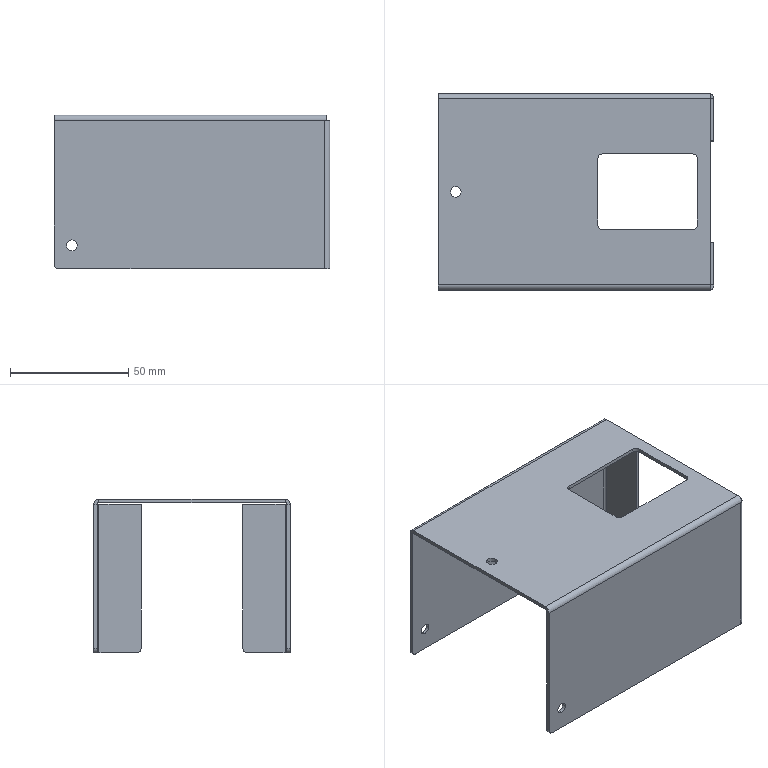Part | STEP file | 01-11 guard plate (Default) | 1 solid | 58 faces | box 116.5 x 83 x 65 mm | volume 37563 mm3 | plane 36 | cylinder 22 | commonest cylinder face diameters 4 x8 4.5 x6 1.473 x4 4.473 x4